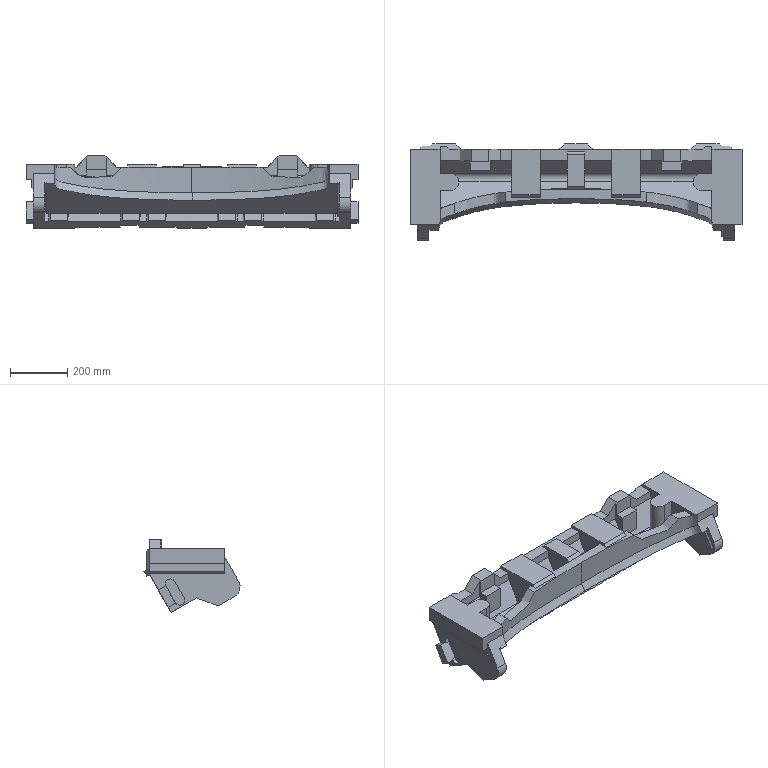Part | NX | features solid 2 | 1 solid | 217 faces | box 1160 x 335.546 x 254.633 mm | volume 29497637 mm3 | plane 187 | cylinder 16 | spline 10 | cone 4 | commonest cylinder face diameters 20 x4 35 x4 40 x4 60 x2 80 x2